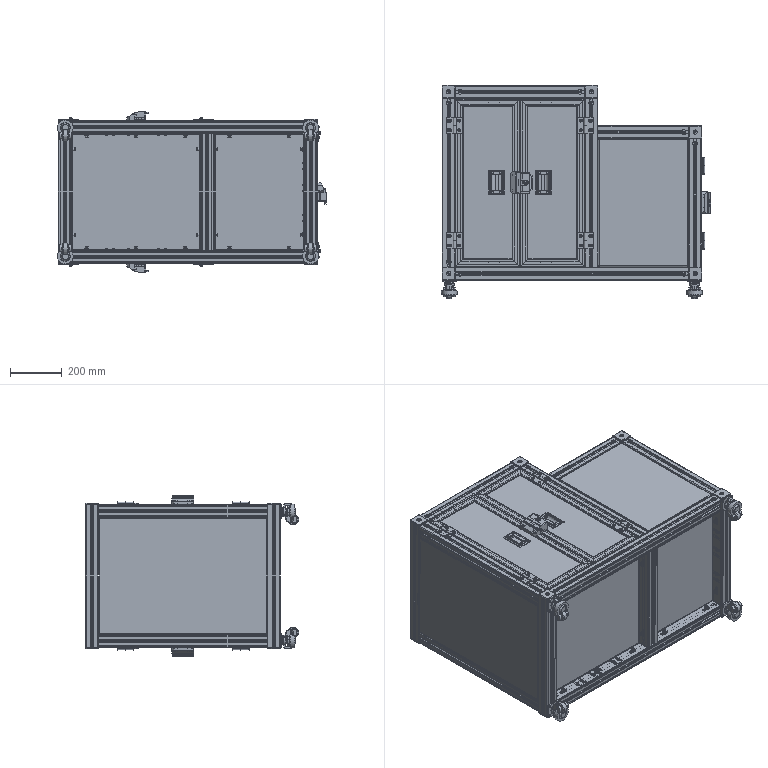Part | NX | features BREP 178 | 1078 solids | 30139 faces | volume 24206027 mm3 | plane 18077 | cylinder 9010 | cone 2248 | torus 614 | sphere 142 | spline 48 | commonest cylinder face diameters 5 x1236 8 x992 2 x914 0.702 x540 6 x418 4 x395